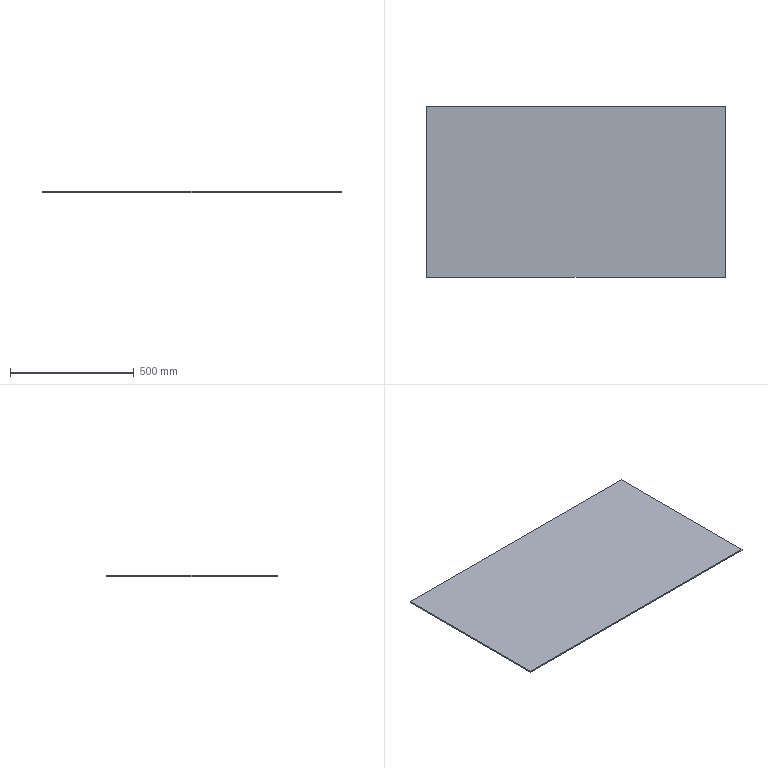Part | SolidWorks | features Extrusion 1, HoleWzd 1 | 1 solid | 6 faces | box 1206 x 690 x 5 mm | volume 4160700 mm3 | plane 6
STEP:
#1=CARTESIAN_POINT('',(603.,-345.,0.));
#2=VERTEX_POINT('',#1);
#3=CARTESIAN_POINT('',(603.,345.,0.));
#4=VERTEX_POINT('',#3);
#5=CARTESIAN_POINT('',(603.,345.,0.));
#6=DIRECTION('',(0.,1.,0.));
#7=VECTOR('',#6,1000.);
#8=LINE('',#5,#7);
#9=EDGE_CURVE('',#2,#4,#8,.T.);
#10=ORIENTED_EDGE('',*,*,#9,.T.);
#11=CARTESIAN_POINT('',(603.,345.,5.));
#12=VERTEX_POINT('',#11);
#13=CARTESIAN_POINT('',(603.,345.,5.));
#14=DIRECTION('',(0.,0.,-1.));
#15=VECTOR('',#14,1000.);
#16=LINE('',#13,#15);
#17=EDGE_CURVE('',#12,#4,#16,.T.);
#18=ORIENTED_EDGE('',*,*,#17,.F.);
#19=CARTESIAN_POINT('',(603.,-345.,5.));
#20=VERTEX_POINT('',#19);
#21=CARTESIAN_POINT('',(603.,345.,5.));
#22=DIRECTION('',(0.,1.,0.));
#23=VECTOR('',#22,1000.);
#24=LINE('',#21,#23);
#25=EDGE_CURVE('',#20,#12,#24,.T.);
#26=ORIENTED_EDGE('',*,*,#25,.F.);
#27=CARTESIAN_POINT('',(603.,-345.,5.));
#28=DIRECTION('',(0.,0.,-1.));
#29=VECTOR('',#28,1000.);
#30=LINE('',#27,#29);
#31=EDGE_CURVE('',#20,#2,#30,.T.);
#32=ORIENTED_EDGE('',*,*,#31,.T.);
#33=EDGE_LOOP('',(#10,#18,#26,#32));
#34=FACE_OUTER_BOUND('',#33,.T.);
#35=CARTESIAN_POINT('',(603.,345.,5.));
#36=DIRECTION('',(-1.,0.,0.));
#37=DIRECTION('',(0.,0.,1.));
#38=AXIS2_PLACEMENT_3D('',#35,#36,#37);
#39=PLANE('',#38);
#40=ADVANCED_FACE('',(#34),#39,.F.);
#41=CARTESIAN_POINT('',(-603.,345.,0.));
#42=VERTEX_POINT('',#41);
#43=CARTESIAN_POINT('',(-603.,345.,0.));
#44=DIRECTION('',(-1.,0.,0.));
#45=VECTOR('',#44,1000.);
#46=LINE('',#43,#45);
#47=EDGE_CURVE('',#4,#42,#46,.T.);
#48=ORIENTED_EDGE('',*,*,#47,.T.);
#49=CARTESIAN_POINT('',(-603.,345.,5.));
#50=VERTEX_POINT('',#49);
#51=CARTESIAN_POINT('',(-603.,345.,5.));
#52=DIRECTION('',(0.,0.,-1.));
#53=VECTOR('',#52,1000.);
#54=LINE('',#51,#53);
#55=EDGE_CURVE('',#50,#42,#54,.T.);
#56=ORIENTED_EDGE('',*,*,#55,.F.);
#57=CARTESIAN_POINT('',(-603.,345.,5.));
#58=DIRECTION('',(-1.,0.,0.));
#59=VECTOR('',#58,1000.);
#60=LINE('',#57,#59);
#61=EDGE_CURVE('',#12,#50,#60,.T.);
#62=ORIENTED_EDGE('',*,*,#61,.F.);
#63=ORIENTED_EDGE('',*,*,#17,.T.);
#64=EDGE_LOOP('',(#48,#56,#62,#63));
#65=FACE_OUTER_BOUND('',#64,.T.);
#66=CARTESIAN_POINT('',(-603.,345.,5.));
#67=DIRECTION('',(0.,-1.,0.));
#68=DIRECTION('',(0.,0.,-1.));
#69=AXIS2_PLACEMENT_3D('',#66,#67,#68);
#70=PLANE('',#69);
#71=ADVANCED_FACE('',(#65),#70,.F.);
#72=CARTESIAN_POINT('',(-603.,-345.,0.));
#73=VERTEX_POINT('',#72);
#74=CARTESIAN_POINT('',(-603.,345.,0.));
#75=DIRECTION('',(0.,-1.,0.));
#76=VECTOR('',#75,1000.);
#77=LINE('',#74,#76);
#78=EDGE_CURVE('',#42,#73,#77,.T.);
#79=ORIENTED_EDGE('',*,*,#78,.T.);
#80=CARTESIAN_POINT('',(-603.,-345.,5.));
#81=VERTEX_POINT('',#80);
#82=CARTESIAN_POINT('',(-603.,-345.,5.));
#83=DIRECTION('',(0.,0.,-1.));
#84=VECTOR('',#83,1000.);
#85=LINE('',#82,#84);
#86=EDGE_CURVE('',#81,#73,#85,.T.);
#87=ORIENTED_EDGE('',*,*,#86,.F.);
#88=CARTESIAN_POINT('',(-603.,345.,5.));
#89=DIRECTION('',(0.,-1.,0.));
#90=VECTOR('',#89,1000.);
#91=LINE('',#88,#90);
#92=EDGE_CURVE('',#50,#81,#91,.T.);
#93=ORIENTED_EDGE('',*,*,#92,.F.);
#94=ORIENTED_EDGE('',*,*,#55,.T.);
#95=EDGE_LOOP('',(#79,#87,#93,#94));
#96=FACE_OUTER_BOUND('',#95,.T.);
#97=CARTESIAN_POINT('',(-603.,345.,5.));
#98=DIRECTION('',(1.,0.,0.));
#99=DIRECTION('',(0.,1.,0.));
#100=AXIS2_PLACEMENT_3D('',#97,#98,#99);
#101=PLANE('',#100);
#102=ADVANCED_FACE('',(#96),#101,.F.);
#103=CARTESIAN_POINT('',(-603.,-345.,0.));
#104=DIRECTION('',(1.,0.,0.));
#105=VECTOR('',#104,1000.);
#106=LINE('',#103,#105);
#107=EDGE_CURVE('',#73,#2,#106,.T.);
#108=ORIENTED_EDGE('',*,*,#107,.T.);
#109=ORIENTED_EDGE('',*,*,#31,.F.);
#110=CARTESIAN_POINT('',(-603.,-345.,5.));
#111=DIRECTION('',(1.,0.,0.));
#112=VECTOR('',#111,1000.);
#113=LINE('',#110,#112);
#114=EDGE_CURVE('',#81,#20,#113,.T.);
#115=ORIENTED_EDGE('',*,*,#114,.F.);
#116=ORIENTED_EDGE('',*,*,#86,.T.);
#117=EDGE_LOOP('',(#108,#109,#115,#116));
#118=FACE_OUTER_BOUND('',#117,.T.);
#119=CARTESIAN_POINT('',(-603.,-345.,5.));
#120=DIRECTION('',(0.,1.,0.));
#121=DIRECTION('',(0.,0.,1.));
#122=AXIS2_PLACEMENT_3D('',#119,#120,#121);
#123=PLANE('',#122);
#124=ADVANCED_FACE('',(#118),#123,.F.);
#125=ORIENTED_EDGE('',*,*,#25,.T.);
#126=ORIENTED_EDGE('',*,*,#61,.T.);
#127=ORIENTED_EDGE('',*,*,#92,.T.);
#128=ORIENTED_EDGE('',*,*,#114,.T.);
#129=EDGE_LOOP('',(#125,#126,#127,#128));
#130=FACE_OUTER_BOUND('',#129,.T.);
#131=CARTESIAN_POINT('',(0.,0.,5.));
#132=DIRECTION('',(0.,0.,1.));
#133=DIRECTION('',(1.,0.,0.));
#134=AXIS2_PLACEMENT_3D('',#131,#132,#133);
#135=PLANE('',#134);
#136=ADVANCED_FACE('',(#130),#135,.T.);
#137=ORIENTED_EDGE('',*,*,#9,.F.);
#138=ORIENTED_EDGE('',*,*,#107,.F.);
#139=ORIENTED_EDGE('',*,*,#78,.F.);
#140=ORIENTED_EDGE('',*,*,#47,.F.);
#141=EDGE_LOOP('',(#137,#138,#139,#140));
#142=FACE_OUTER_BOUND('',#141,.T.);
#143=CARTESIAN_POINT('',(0.,0.,0.));
#144=DIRECTION('',(0.,0.,1.));
#145=DIRECTION('',(1.,0.,0.));
#146=AXIS2_PLACEMENT_3D('',#143,#144,#145);
#147=PLANE('',#146);
#148=ADVANCED_FACE('',(#142),#147,.F.);
#149=CLOSED_SHELL('',(#40,#71,#102,#124,#136,#148));
#150=MANIFOLD_SOLID_BREP('',#149);
#151=CARTESIAN_POINT('',(0.,0.,0.));
#152=DIRECTION('',(0.,0.,1.));
#153=DIRECTION('',(1.,0.,0.));
#154=AXIS2_PLACEMENT_3D('',#151,#152,#153);
#155=(LENGTH_UNIT()NAMED_UNIT(*)SI_UNIT(.MILLI.,.METRE.));
#156=UNCERTAINTY_MEASURE_WITH_UNIT(LENGTH_MEASURE(0.00001),#155,'','');
#157=(NAMED_UNIT(*)PLANE_ANGLE_UNIT()SI_UNIT($,.RADIAN.));
#158=(NAMED_UNIT(*)SI_UNIT($,.STERADIAN.)SOLID_ANGLE_UNIT());
#159=(GEOMETRIC_REPRESENTATION_CONTEXT(3)GLOBAL_UNCERTAINTY_ASSIGNED_CONTEXT((#156))GLOBAL_UNIT_ASSIGNED_CONTEXT((#155,#157,#158))REPRESENTATION_CONTEXT('',''));
#160=ADVANCED_BREP_SHAPE_REPRESENTATION('',(#150,#154),#159);